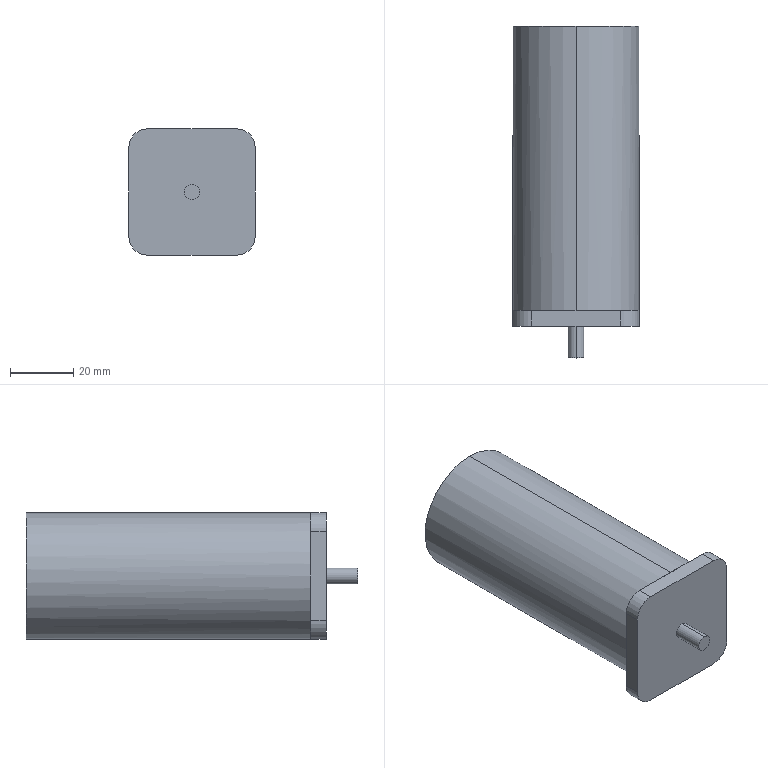Part | SolidWorks | features BaseBody 1 | 1 solid | 19 faces | box 40 x 105 x 40 mm | volume 121139 mm3 | plane 11 | cylinder 8 | commonest cylinder face diameters 12 x4 5 x2 40 x2
STEP:
#1=CARTESIAN_POINT('',(-147.5,290.,154.5));
#2=VERTEX_POINT('',#1);
#3=CARTESIAN_POINT('',(-147.5,290.,149.5));
#4=VERTEX_POINT('',#3);
#5=CARTESIAN_POINT('',(-147.5,290.,152.));
#6=DIRECTION('',(0.,-1.,0.));
#7=DIRECTION('',(0.,0.,-1.));
#8=AXIS2_PLACEMENT_3D('',#5,#6,#7);
#9=CIRCLE('',#8,2.5);
#10=EDGE_CURVE('',#2,#4,#9,.T.);
#11=ORIENTED_EDGE('',*,*,#10,.F.);
#12=CARTESIAN_POINT('',(-147.5,300.,154.5));
#13=VERTEX_POINT('',#12);
#14=CARTESIAN_POINT('',(-147.5,292.,154.5));
#15=DIRECTION('',(0.,1.,0.));
#16=VECTOR('',#15,1000.);
#17=LINE('',#14,#16);
#18=EDGE_CURVE('',#2,#13,#17,.T.);
#19=ORIENTED_EDGE('',*,*,#18,.T.);
#20=CARTESIAN_POINT('',(-147.5,300.,149.5));
#21=VERTEX_POINT('',#20);
#22=CARTESIAN_POINT('',(-147.5,300.,152.));
#23=DIRECTION('',(0.,-1.,0.));
#24=DIRECTION('',(1.,0.,0.));
#25=AXIS2_PLACEMENT_3D('',#22,#23,#24);
#26=CIRCLE('',#25,2.5);
#27=EDGE_CURVE('',#13,#21,#26,.T.);
#28=ORIENTED_EDGE('',*,*,#27,.T.);
#29=CARTESIAN_POINT('',(-147.5,292.,149.5));
#30=DIRECTION('',(0.,1.,0.));
#31=VECTOR('',#30,1000.);
#32=LINE('',#29,#31);
#33=EDGE_CURVE('',#4,#21,#32,.T.);
#34=ORIENTED_EDGE('',*,*,#33,.F.);
#35=EDGE_LOOP('',(#11,#19,#28,#34));
#36=FACE_OUTER_BOUND('',#35,.T.);
#37=CARTESIAN_POINT('',(-147.5,292.,152.));
#38=DIRECTION('',(0.,1.,0.));
#39=DIRECTION('',(0.,0.,-1.));
#40=AXIS2_PLACEMENT_3D('',#37,#38,#39);
#41=CYLINDRICAL_SURFACE('',#40,2.5);
#42=ADVANCED_FACE('',(#36),#41,.T.);
#43=CARTESIAN_POINT('',(-147.5,395.,132.));
#44=VERTEX_POINT('',#43);
#45=CARTESIAN_POINT('',(-147.5,395.,172.));
#46=VERTEX_POINT('',#45);
#47=CARTESIAN_POINT('',(-147.5,395.,152.));
#48=DIRECTION('',(0.,1.,0.));
#49=DIRECTION('',(1.,0.,0.));
#50=AXIS2_PLACEMENT_3D('',#47,#48,#49);
#51=CIRCLE('',#50,20.);
#52=EDGE_CURVE('',#44,#46,#51,.T.);
#53=ORIENTED_EDGE('',*,*,#52,.F.);
#54=CARTESIAN_POINT('',(-147.5,305.,132.));
#55=VERTEX_POINT('',#54);
#56=CARTESIAN_POINT('',(-147.5,395.,132.));
#57=DIRECTION('',(0.,-1.,0.));
#58=VECTOR('',#57,1000.);
#59=LINE('',#56,#58);
#60=EDGE_CURVE('',#44,#55,#59,.T.);
#61=ORIENTED_EDGE('',*,*,#60,.T.);
#62=CARTESIAN_POINT('',(-167.5,305.,152.));
#63=VERTEX_POINT('',#62);
#64=CARTESIAN_POINT('',(-147.5,305.,152.));
#65=DIRECTION('',(0.,1.,0.));
#66=DIRECTION('',(1.,0.,0.));
#67=AXIS2_PLACEMENT_3D('',#64,#65,#66);
#68=CIRCLE('',#67,20.);
#69=EDGE_CURVE('',#55,#63,#68,.T.);
#70=ORIENTED_EDGE('',*,*,#69,.T.);
#71=CARTESIAN_POINT('',(-147.5,305.,172.));
#72=VERTEX_POINT('',#71);
#73=CARTESIAN_POINT('',(-147.5,305.,152.));
#74=DIRECTION('',(0.,1.,0.));
#75=DIRECTION('',(1.,0.,0.));
#76=AXIS2_PLACEMENT_3D('',#73,#74,#75);
#77=CIRCLE('',#76,20.);
#78=EDGE_CURVE('',#63,#72,#77,.T.);
#79=ORIENTED_EDGE('',*,*,#78,.T.);
#80=CARTESIAN_POINT('',(-147.5,395.,172.));
#81=DIRECTION('',(0.,-1.,0.));
#82=VECTOR('',#81,1000.);
#83=LINE('',#80,#82);
#84=EDGE_CURVE('',#46,#72,#83,.T.);
#85=ORIENTED_EDGE('',*,*,#84,.F.);
#86=EDGE_LOOP('',(#53,#61,#70,#79,#85));
#87=FACE_OUTER_BOUND('',#86,.T.);
#88=CARTESIAN_POINT('',(-147.5,395.,152.));
#89=DIRECTION('',(0.,-1.,0.));
#90=DIRECTION('',(0.,0.,1.));
#91=AXIS2_PLACEMENT_3D('',#88,#89,#90);
#92=CYLINDRICAL_SURFACE('',#91,20.);
#93=ADVANCED_FACE('',(#87),#92,.T.);
#94=CARTESIAN_POINT('',(-127.5,305.,152.));
#95=VERTEX_POINT('',#94);
#96=CARTESIAN_POINT('',(-127.5,305.,138.));
#97=VERTEX_POINT('',#96);
#98=CARTESIAN_POINT('',(-127.5,305.,172.));
#99=DIRECTION('',(0.,0.,-1.));
#100=VECTOR('',#99,1000.);
#101=LINE('',#98,#100);
#102=EDGE_CURVE('',#95,#97,#101,.T.);
#103=ORIENTED_EDGE('',*,*,#102,.T.);
#104=CARTESIAN_POINT('',(-133.5,305.,132.));
#105=VERTEX_POINT('',#104);
#106=CARTESIAN_POINT('',(-133.5,305.,138.));
#107=DIRECTION('',(0.,1.,0.));
#108=DIRECTION('',(0.,0.,1.));
#109=AXIS2_PLACEMENT_3D('',#106,#107,#108);
#110=CIRCLE('',#109,6.);
#111=EDGE_CURVE('',#97,#105,#110,.T.);
#112=ORIENTED_EDGE('',*,*,#111,.T.);
#113=CARTESIAN_POINT('',(-127.5,305.,132.));
#114=DIRECTION('',(-1.,0.,0.));
#115=VECTOR('',#114,1000.);
#116=LINE('',#113,#115);
#117=EDGE_CURVE('',#105,#55,#116,.T.);
#118=ORIENTED_EDGE('',*,*,#117,.T.);
#119=CARTESIAN_POINT('',(-147.5,305.,152.));
#120=DIRECTION('',(0.,1.,0.));
#121=DIRECTION('',(1.,0.,0.));
#122=AXIS2_PLACEMENT_3D('',#119,#120,#121);
#123=CIRCLE('',#122,20.);
#124=EDGE_CURVE('',#95,#55,#123,.T.);
#125=ORIENTED_EDGE('',*,*,#124,.F.);
#126=EDGE_LOOP('',(#103,#112,#118,#125));
#127=FACE_OUTER_BOUND('',#126,.T.);
#128=CARTESIAN_POINT('',(2.5,305.,12.));
#129=DIRECTION('',(0.,1.,0.));
#130=DIRECTION('',(0.,0.,-1.));
#131=AXIS2_PLACEMENT_3D('',#128,#129,#130);
#132=PLANE('',#131);
#133=ADVANCED_FACE('',(#127),#132,.T.);
#134=CARTESIAN_POINT('',(-161.5,305.,132.));
#135=VERTEX_POINT('',#134);
#136=CARTESIAN_POINT('',(-127.5,305.,132.));
#137=DIRECTION('',(-1.,0.,0.));
#138=VECTOR('',#137,1000.);
#139=LINE('',#136,#138);
#140=EDGE_CURVE('',#55,#135,#139,.T.);
#141=ORIENTED_EDGE('',*,*,#140,.T.);
#142=CARTESIAN_POINT('',(-167.5,305.,138.));
#143=VERTEX_POINT('',#142);
#144=CARTESIAN_POINT('',(-161.5,305.,138.));
#145=DIRECTION('',(0.,1.,0.));
#146=DIRECTION('',(0.,0.,1.));
#147=AXIS2_PLACEMENT_3D('',#144,#145,#146);
#148=CIRCLE('',#147,6.);
#149=EDGE_CURVE('',#135,#143,#148,.T.);
#150=ORIENTED_EDGE('',*,*,#149,.T.);
#151=CARTESIAN_POINT('',(-167.5,305.,132.));
#152=DIRECTION('',(0.,0.,1.));
#153=VECTOR('',#152,1000.);
#154=LINE('',#151,#153);
#155=EDGE_CURVE('',#143,#63,#154,.T.);
#156=ORIENTED_EDGE('',*,*,#155,.T.);
#157=ORIENTED_EDGE('',*,*,#69,.F.);
#158=EDGE_LOOP('',(#141,#150,#156,#157));
#159=FACE_OUTER_BOUND('',#158,.T.);
#160=CARTESIAN_POINT('',(2.5,305.,12.));
#161=DIRECTION('',(0.,1.,0.));
#162=DIRECTION('',(0.,0.,-1.));
#163=AXIS2_PLACEMENT_3D('',#160,#161,#162);
#164=PLANE('',#163);
#165=ADVANCED_FACE('',(#159),#164,.T.);
#166=CARTESIAN_POINT('',(-167.5,305.,166.));
#167=VERTEX_POINT('',#166);
#168=CARTESIAN_POINT('',(-167.5,305.,132.));
#169=DIRECTION('',(0.,0.,1.));
#170=VECTOR('',#169,1000.);
#171=LINE('',#168,#170);
#172=EDGE_CURVE('',#63,#167,#171,.T.);
#173=ORIENTED_EDGE('',*,*,#172,.T.);
#174=CARTESIAN_POINT('',(-161.5,305.,172.));
#175=VERTEX_POINT('',#174);
#176=CARTESIAN_POINT('',(-161.5,305.,166.));
#177=DIRECTION('',(0.,1.,0.));
#178=DIRECTION('',(0.,0.,1.));
#179=AXIS2_PLACEMENT_3D('',#176,#177,#178);
#180=CIRCLE('',#179,6.);
#181=EDGE_CURVE('',#167,#175,#180,.T.);
#182=ORIENTED_EDGE('',*,*,#181,.T.);
#183=CARTESIAN_POINT('',(-167.5,305.,172.));
#184=DIRECTION('',(1.,0.,0.));
#185=VECTOR('',#184,1000.);
#186=LINE('',#183,#185);
#187=EDGE_CURVE('',#175,#72,#186,.T.);
#188=ORIENTED_EDGE('',*,*,#187,.T.);
#189=ORIENTED_EDGE('',*,*,#78,.F.);
#190=EDGE_LOOP('',(#173,#182,#188,#189));
#191=FACE_OUTER_BOUND('',#190,.T.);
#192=CARTESIAN_POINT('',(2.5,305.,12.));
#193=DIRECTION('',(0.,1.,0.));
#194=DIRECTION('',(0.,0.,-1.));
#195=AXIS2_PLACEMENT_3D('',#192,#193,#194);
#196=PLANE('',#195);
#197=ADVANCED_FACE('',(#191),#196,.T.);
#198=CARTESIAN_POINT('',(-161.5,300.,172.));
#199=VERTEX_POINT('',#198);
#200=CARTESIAN_POINT('',(-133.5,300.,172.));
#201=VERTEX_POINT('',#200);
#202=CARTESIAN_POINT('',(-167.5,300.,172.));
#203=DIRECTION('',(1.,0.,0.));
#204=VECTOR('',#203,1000.);
#205=LINE('',#202,#204);
#206=EDGE_CURVE('',#199,#201,#205,.T.);
#207=ORIENTED_EDGE('',*,*,#206,.T.);
#208=CARTESIAN_POINT('',(-133.5,305.,172.));
#209=VERTEX_POINT('',#208);
#210=CARTESIAN_POINT('',(-133.5,305.,172.));
#211=DIRECTION('',(0.,1.,0.));
#212=VECTOR('',#211,1000.);
#213=LINE('',#210,#212);
#214=EDGE_CURVE('',#201,#209,#213,.T.);
#215=ORIENTED_EDGE('',*,*,#214,.T.);
#216=CARTESIAN_POINT('',(-167.5,305.,172.));
#217=DIRECTION('',(1.,0.,0.));
#218=VECTOR('',#217,1000.);
#219=LINE('',#216,#218);
#220=EDGE_CURVE('',#72,#209,#219,.T.);
#221=ORIENTED_EDGE('',*,*,#220,.F.);
#222=ORIENTED_EDGE('',*,*,#187,.F.);
#223=CARTESIAN_POINT('',(-161.5,305.,172.));
#224=DIRECTION('',(0.,-1.,0.));
#225=VECTOR('',#224,1000.);
#226=LINE('',#223,#225);
#227=EDGE_CURVE('',#175,#199,#226,.T.);
#228=ORIENTED_EDGE('',*,*,#227,.T.);
#229=EDGE_LOOP('',(#207,#215,#221,#222,#228));
#230=FACE_OUTER_BOUND('',#229,.T.);
#231=CARTESIAN_POINT('',(-167.5,305.,172.));
#232=DIRECTION('',(0.,0.,-1.));
#233=DIRECTION('',(0.,-1.,0.));
#234=AXIS2_PLACEMENT_3D('',#231,#232,#233);
#235=PLANE('',#234);
#236=ADVANCED_FACE('',(#230),#235,.F.);
#237=CARTESIAN_POINT('',(-127.5,305.,166.));
#238=VERTEX_POINT('',#237);
#239=CARTESIAN_POINT('',(-127.5,305.,172.));
#240=DIRECTION('',(0.,0.,-1.));
#241=VECTOR('',#240,1000.);
#242=LINE('',#239,#241);
#243=EDGE_CURVE('',#238,#95,#242,.T.);
#244=ORIENTED_EDGE('',*,*,#243,.F.);
#245=CARTESIAN_POINT('',(-127.5,300.,166.));
#246=VERTEX_POINT('',#245);
#247=CARTESIAN_POINT('',(-127.5,305.,166.));
#248=DIRECTION('',(0.,-1.,0.));
#249=VECTOR('',#248,1000.);
#250=LINE('',#247,#249);
#251=EDGE_CURVE('',#238,#246,#250,.T.);
#252=ORIENTED_EDGE('',*,*,#251,.T.);
#253=CARTESIAN_POINT('',(-127.5,300.,138.));
#254=VERTEX_POINT('',#253);
#255=CARTESIAN_POINT('',(-127.5,300.,172.));
#256=DIRECTION('',(0.,0.,-1.));
#257=VECTOR('',#256,1000.);
#258=LINE('',#255,#257);
#259=EDGE_CURVE('',#246,#254,#258,.T.);
#260=ORIENTED_EDGE('',*,*,#259,.T.);
#261=CARTESIAN_POINT('',(-127.5,305.,138.));
#262=DIRECTION('',(0.,1.,0.));
#263=VECTOR('',#262,1000.);
#264=LINE('',#261,#263);
#265=EDGE_CURVE('',#254,#97,#264,.T.);
#266=ORIENTED_EDGE('',*,*,#265,.T.);
#267=ORIENTED_EDGE('',*,*,#102,.F.);
#268=EDGE_LOOP('',(#244,#252,#260,#266,#267));
#269=FACE_OUTER_BOUND('',#268,.T.);
#270=CARTESIAN_POINT('',(-127.5,305.,172.));
#271=DIRECTION('',(-1.,0.,0.));
#272=DIRECTION('',(0.,0.,-1.));
#273=AXIS2_PLACEMENT_3D('',#270,#271,#272);
#274=PLANE('',#273);
#275=ADVANCED_FACE('',(#269),#274,.F.);
#276=CARTESIAN_POINT('',(-133.5,300.,132.));
#277=VERTEX_POINT('',#276);
#278=CARTESIAN_POINT('',(-161.5,300.,132.));
#279=VERTEX_POINT('',#278);
#280=CARTESIAN_POINT('',(-127.5,300.,132.));
#281=DIRECTION('',(-1.,0.,0.));
#282=VECTOR('',#281,1000.);
#283=LINE('',#280,#282);
#284=EDGE_CURVE('',#277,#279,#283,.T.);
#285=ORIENTED_EDGE('',*,*,#284,.T.);
#286=CARTESIAN_POINT('',(-161.5,305.,132.));
#287=DIRECTION('',(0.,1.,0.));
#288=VECTOR('',#287,1000.);
#289=LINE('',#286,#288);
#290=EDGE_CURVE('',#279,#135,#289,.T.);
#291=ORIENTED_EDGE('',*,*,#290,.T.);
#292=ORIENTED_EDGE('',*,*,#140,.F.);
#293=ORIENTED_EDGE('',*,*,#117,.F.);
#294=CARTESIAN_POINT('',(-133.5,305.,132.));
#295=DIRECTION('',(0.,-1.,0.));
#296=VECTOR('',#295,1000.);
#297=LINE('',#294,#296);
#298=EDGE_CURVE('',#105,#277,#297,.T.);
#299=ORIENTED_EDGE('',*,*,#298,.T.);
#300=EDGE_LOOP('',(#285,#291,#292,#293,#299));
#301=FACE_OUTER_BOUND('',#300,.T.);
#302=CARTESIAN_POINT('',(-127.5,305.,132.));
#303=DIRECTION('',(0.,0.,1.));
#304=DIRECTION('',(0.,1.,0.));
#305=AXIS2_PLACEMENT_3D('',#302,#303,#304);
#306=PLANE('',#305);
#307=ADVANCED_FACE('',(#301),#306,.F.);
#308=CARTESIAN_POINT('',(-167.5,300.,138.));
#309=VERTEX_POINT('',#308);
#310=CARTESIAN_POINT('',(-167.5,300.,166.));
#311=VERTEX_POINT('',#310);
#312=CARTESIAN_POINT('',(-167.5,300.,132.));
#313=DIRECTION('',(0.,0.,1.));
#314=VECTOR('',#313,1000.);
#315=LINE('',#312,#314);
#316=EDGE_CURVE('',#309,#311,#315,.T.);
#317=ORIENTED_EDGE('',*,*,#316,.T.);
#318=CARTESIAN_POINT('',(-167.5,305.,166.));
#319=DIRECTION('',(0.,1.,0.));
#320=VECTOR('',#319,1000.);
#321=LINE('',#318,#320);
#322=EDGE_CURVE('',#311,#167,#321,.T.);
#323=ORIENTED_EDGE('',*,*,#322,.T.);
#324=ORIENTED_EDGE('',*,*,#172,.F.);
#325=ORIENTED_EDGE('',*,*,#155,.F.);
#326=CARTESIAN_POINT('',(-167.5,305.,138.));
#327=DIRECTION('',(0.,-1.,0.));
#328=VECTOR('',#327,1000.);
#329=LINE('',#326,#328);
#330=EDGE_CURVE('',#143,#309,#329,.T.);
#331=ORIENTED_EDGE('',*,*,#330,.T.);
#332=EDGE_LOOP('',(#317,#323,#324,#325,#331));
#333=FACE_OUTER_BOUND('',#332,.T.);
#334=CARTESIAN_POINT('',(-167.5,305.,132.));
#335=DIRECTION('',(1.,0.,0.));
#336=DIRECTION('',(0.,0.,1.));
#337=AXIS2_PLACEMENT_3D('',#334,#335,#336);
#338=PLANE('',#337);
#339=ADVANCED_FACE('',(#333),#338,.F.);
#340=ORIENTED_EDGE('',*,*,#220,.T.);
#341=CARTESIAN_POINT('',(-133.5,305.,166.));
#342=DIRECTION('',(0.,1.,0.));
#343=DIRECTION('',(0.,0.,1.));
#344=AXIS2_PLACEMENT_3D('',#341,#342,#343);
#345=CIRCLE('',#344,6.);
#346=EDGE_CURVE('',#209,#238,#345,.T.);
#347=ORIENTED_EDGE('',*,*,#346,.T.);
#348=ORIENTED_EDGE('',*,*,#243,.T.);
#349=CARTESIAN_POINT('',(-147.5,305.,152.));
#350=DIRECTION('',(0.,1.,0.));
#351=DIRECTION('',(1.,0.,0.));
#352=AXIS2_PLACEMENT_3D('',#349,#350,#351);
#353=CIRCLE('',#352,20.);
#354=EDGE_CURVE('',#72,#95,#353,.T.);
#355=ORIENTED_EDGE('',*,*,#354,.F.);
#356=EDGE_LOOP('',(#340,#347,#348,#355));
#357=FACE_OUTER_BOUND('',#356,.T.);
#358=CARTESIAN_POINT('',(2.5,305.,12.));
#359=DIRECTION('',(0.,1.,0.));
#360=DIRECTION('',(0.,0.,-1.));
#361=AXIS2_PLACEMENT_3D('',#358,#359,#360);
#362=PLANE('',#361);
#363=ADVANCED_FACE('',(#357),#362,.T.);
#364=CARTESIAN_POINT('',(-147.5,300.,152.));
#365=DIRECTION('',(0.,-1.,0.));
#366=DIRECTION('',(1.,0.,0.));
#367=AXIS2_PLACEMENT_3D('',#364,#365,#366);
#368=CIRCLE('',#367,2.5);
#369=EDGE_CURVE('',#21,#13,#368,.T.);
#370=ORIENTED_EDGE('',*,*,#369,.F.);
#371=ORIENTED_EDGE('',*,*,#27,.F.);
#372=EDGE_LOOP('',(#370,#371));
#373=FACE_BOUND('',#372,.T.);
#374=ORIENTED_EDGE('',*,*,#259,.F.);
#375=CARTESIAN_POINT('',(-133.5,300.,166.));
#376=DIRECTION('',(0.,-1.,0.));
#377=DIRECTION('',(0.,0.,1.));
#378=AXIS2_PLACEMENT_3D('',#375,#376,#377);
#379=CIRCLE('',#378,6.);
#380=EDGE_CURVE('',#246,#201,#379,.T.);
#381=ORIENTED_EDGE('',*,*,#380,.T.);
#382=ORIENTED_EDGE('',*,*,#206,.F.);
#383=CARTESIAN_POINT('',(-161.5,300.,166.));
#384=DIRECTION('',(0.,-1.,0.));
#385=DIRECTION('',(0.,0.,1.));
#386=AXIS2_PLACEMENT_3D('',#383,#384,#385);
#387=CIRCLE('',#386,6.);
#388=EDGE_CURVE('',#199,#311,#387,.T.);
#389=ORIENTED_EDGE('',*,*,#388,.T.);
#390=ORIENTED_EDGE('',*,*,#316,.F.);
#391=CARTESIAN_POINT('',(-161.5,300.,138.));
#392=DIRECTION('',(0.,-1.,0.));
#393=DIRECTION('',(0.,0.,1.));
#394=AXIS2_PLACEMENT_3D('',#391,#392,#393);
#395=CIRCLE('',#394,6.);
#396=EDGE_CURVE('',#309,#279,#395,.T.);
#397=ORIENTED_EDGE('',*,*,#396,.T.);
#398=ORIENTED_EDGE('',*,*,#284,.F.);
#399=CARTESIAN_POINT('',(-133.5,300.,138.));
#400=DIRECTION('',(0.,-1.,0.));
#401=DIRECTION('',(0.,0.,1.));
#402=AXIS2_PLACEMENT_3D('',#399,#400,#401);
#403=CIRCLE('',#402,6.);
#404=EDGE_CURVE('',#277,#254,#403,.T.);
#405=ORIENTED_EDGE('',*,*,#404,.T.);
#406=EDGE_LOOP('',(#374,#381,#382,#389,#390,#397,#398,#405));
#407=FACE_OUTER_BOUND('',#406,.T.);
#408=CARTESIAN_POINT('',(2.5,300.,12.));
#409=DIRECTION('',(0.,1.,0.));
#410=DIRECTION('',(0.,0.,-1.));
#411=AXIS2_PLACEMENT_3D('',#408,#409,#410);
#412=PLANE('',#411);
#413=ADVANCED_FACE('',(#373,#407),#412,.F.);
#414=ORIENTED_EDGE('',*,*,#60,.F.);
#415=CARTESIAN_POINT('',(-147.5,395.,152.));
#416=DIRECTION('',(0.,1.,0.));
#417=DIRECTION('',(1.,0.,0.));
#418=AXIS2_PLACEMENT_3D('',#415,#416,#417);
#419=CIRCLE('',#418,20.);
#420=EDGE_CURVE('',#46,#44,#419,.T.);
#421=ORIENTED_EDGE('',*,*,#420,.F.);
#422=ORIENTED_EDGE('',*,*,#84,.T.);
#423=ORIENTED_EDGE('',*,*,#354,.T.);
#424=ORIENTED_EDGE('',*,*,#124,.T.);
#425=EDGE_LOOP('',(#414,#421,#422,#423,#424));
#426=FACE_OUTER_BOUND('',#425,.T.);
#427=CARTESIAN_POINT('',(-147.5,395.,152.));
#428=DIRECTION('',(0.,-1.,0.));
#429=DIRECTION('',(0.,0.,1.));
#430=AXIS2_PLACEMENT_3D('',#427,#428,#429);
#431=CYLINDRICAL_SURFACE('',#430,20.);
#432=ADVANCED_FACE('',(#426),#431,.T.);
#433=ORIENTED_EDGE('',*,*,#420,.T.);
#434=ORIENTED_EDGE('',*,*,#52,.T.);
#435=EDGE_LOOP('',(#433,#434));
#436=FACE_OUTER_BOUND('',#435,.T.);
#437=CARTESIAN_POINT('',(-147.5,395.,152.));
#438=DIRECTION('',(0.,1.,0.));
#439=DIRECTION('',(0.,0.,-1.));
#440=AXIS2_PLACEMENT_3D('',#437,#438,#439);
#441=PLANE('',#440);
#442=ADVANCED_FACE('',(#436),#441,.T.);
#443=ORIENTED_EDGE('',*,*,#18,.F.);
#444=CARTESIAN_POINT('',(-147.5,290.,152.));
#445=DIRECTION('',(0.,-1.,0.));
#446=DIRECTION('',(0.,0.,-1.));
#447=AXIS2_PLACEMENT_3D('',#444,#445,#446);
#448=CIRCLE('',#447,2.5);
#449=EDGE_CURVE('',#4,#2,#448,.T.);
#450=ORIENTED_EDGE('',*,*,#449,.F.);
#451=ORIENTED_EDGE('',*,*,#33,.T.);
#452=ORIENTED_EDGE('',*,*,#369,.T.);
#453=EDGE_LOOP('',(#443,#450,#451,#452));
#454=FACE_OUTER_BOUND('',#453,.T.);
#455=CARTESIAN_POINT('',(-147.5,292.,152.));
#456=DIRECTION('',(0.,1.,0.));
#457=DIRECTION('',(0.,0.,-1.));
#458=AXIS2_PLACEMENT_3D('',#455,#456,#457);
#459=CYLINDRICAL_SURFACE('',#458,2.5);
#460=ADVANCED_FACE('',(#454),#459,.T.);
#461=ORIENTED_EDGE('',*,*,#449,.T.);
#462=ORIENTED_EDGE('',*,*,#10,.T.);
#463=EDGE_LOOP('',(#461,#462));
#464=FACE_OUTER_BOUND('',#463,.T.);
#465=CARTESIAN_POINT('',(-147.5,290.,152.));
#466=DIRECTION('',(0.,-1.,0.));
#467=DIRECTION('',(0.,0.,1.));
#468=AXIS2_PLACEMENT_3D('',#465,#466,#467);
#469=PLANE('',#468);
#470=ADVANCED_FACE('',(#464),#469,.T.);
#471=ORIENTED_EDGE('',*,*,#346,.F.);
#472=ORIENTED_EDGE('',*,*,#214,.F.);
#473=ORIENTED_EDGE('',*,*,#380,.F.);
#474=ORIENTED_EDGE('',*,*,#251,.F.);
#475=EDGE_LOOP('',(#471,#472,#473,#474));
#476=FACE_OUTER_BOUND('',#475,.T.);
#477=CARTESIAN_POINT('',(-133.5,305.,166.));
#478=DIRECTION('',(0.,-1.,0.));
#479=DIRECTION('',(0.,0.,-1.));
#480=AXIS2_PLACEMENT_3D('',#477,#478,#479);
#481=CYLINDRICAL_SURFACE('',#480,6.);
#482=ADVANCED_FACE('',(#476),#481,.T.);
#483=ORIENTED_EDGE('',*,*,#181,.F.);
#484=ORIENTED_EDGE('',*,*,#322,.F.);
#485=ORIENTED_EDGE('',*,*,#388,.F.);
#486=ORIENTED_EDGE('',*,*,#227,.F.);
#487=EDGE_LOOP('',(#483,#484,#485,#486));
#488=FACE_OUTER_BOUND('',#487,.T.);
#489=CARTESIAN_POINT('',(-161.5,305.,166.));
#490=DIRECTION('',(0.,-1.,0.));
#491=DIRECTION('',(0.,0.,-1.));
#492=AXIS2_PLACEMENT_3D('',#489,#490,#491);
#493=CYLINDRICAL_SURFACE('',#492,6.);
#494=ADVANCED_FACE('',(#488),#493,.T.);
#495=ORIENTED_EDGE('',*,*,#149,.F.);
#496=ORIENTED_EDGE('',*,*,#290,.F.);
#497=ORIENTED_EDGE('',*,*,#396,.F.);
#498=ORIENTED_EDGE('',*,*,#330,.F.);
#499=EDGE_LOOP('',(#495,#496,#497,#498));
#500=FACE_OUTER_BOUND('',#499,.T.);
#501=CARTESIAN_POINT('',(-161.5,305.,138.));
#502=DIRECTION('',(0.,-1.,0.));
#503=DIRECTION('',(0.,0.,-1.));
#504=AXIS2_PLACEMENT_3D('',#501,#502,#503);
#505=CYLINDRICAL_SURFACE('',#504,6.);
#506=ADVANCED_FACE('',(#500),#505,.T.);
#507=ORIENTED_EDGE('',*,*,#111,.F.);
#508=ORIENTED_EDGE('',*,*,#265,.F.);
#509=ORIENTED_EDGE('',*,*,#404,.F.);
#510=ORIENTED_EDGE('',*,*,#298,.F.);
#511=EDGE_LOOP('',(#507,#508,#509,#510));
#512=FACE_OUTER_BOUND('',#511,.T.);
#513=CARTESIAN_POINT('',(-133.5,305.,138.));
#514=DIRECTION('',(0.,-1.,0.));
#515=DIRECTION('',(0.,0.,-1.));
#516=AXIS2_PLACEMENT_3D('',#513,#514,#515);
#517=CYLINDRICAL_SURFACE('',#516,6.);
#518=ADVANCED_FACE('',(#512),#517,.T.);
#519=CLOSED_SHELL('',(#42,#93,#133,#165,#197,#236,#275,#307,#339,#363,#413,#432,#442,#460,#470,#482,#494,#506,#518));
#520=MANIFOLD_SOLID_BREP('',#519);
#521=CARTESIAN_POINT('',(0.,0.,0.));
#522=DIRECTION('',(0.,0.,1.));
#523=DIRECTION('',(1.,0.,0.));
#524=AXIS2_PLACEMENT_3D('',#521,#522,#523);
#525=(LENGTH_UNIT()NAMED_UNIT(*)SI_UNIT(.MILLI.,.METRE.));
#526=UNCERTAINTY_MEASURE_WITH_UNIT(LENGTH_MEASURE(0.00001),#525,'','');
#527=(NAMED_UNIT(*)PLANE_ANGLE_UNIT()SI_UNIT($,.RADIAN.));
#528=(NAMED_UNIT(*)SI_UNIT($,.STERADIAN.)SOLID_ANGLE_UNIT());
#529=(GEOMETRIC_REPRESENTATION_CONTEXT(3)GLOBAL_UNCERTAINTY_ASSIGNED_CONTEXT((#526))GLOBAL_UNIT_ASSIGNED_CONTEXT((#525,#527,#528))REPRESENTATION_CONTEXT('',''));
#530=ADVANCED_BREP_SHAPE_REPRESENTATION('',(#520,#524),#529);